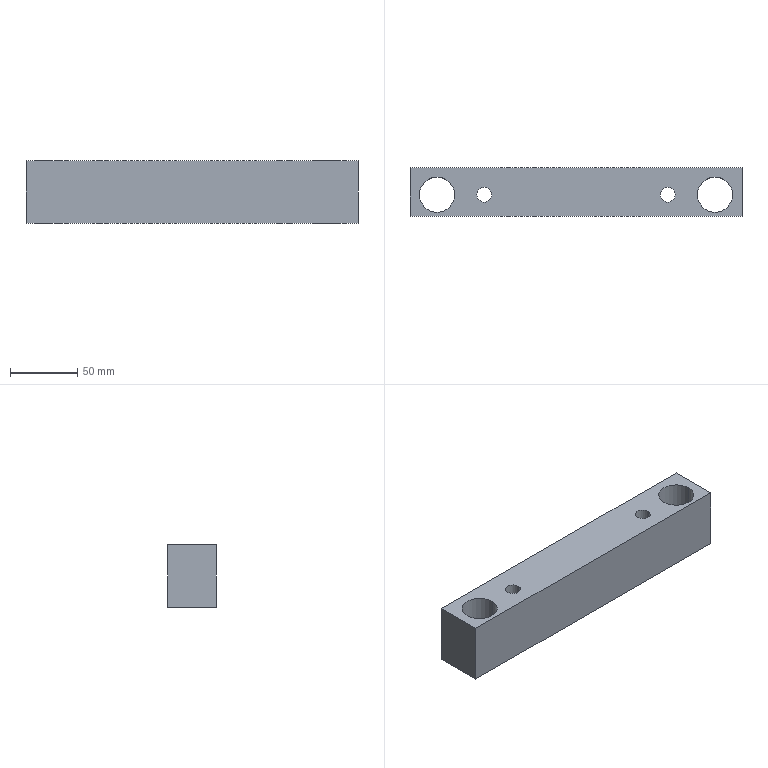Part | STEP file | 5 | 1 solid | 14 faces | box 246 x 36 x 46 mm | volume 349787 mm3 | cylinder 8 | plane 6 | commonest cylinder face diameters 11 x4 26 x4
STEP:
#1=CARTESIAN_POINT('',(0.,0.,0.));
#2=DIRECTION('',(0.,0.,1.));
#3=DIRECTION('',(1.,0.,0.));
#4=AXIS2_PLACEMENT_3D('',#1,#2,#3);
#5=CARTESIAN_POINT('',(116.,78.,22.));
#6=VERTEX_POINT('',#5);
#7=CARTESIAN_POINT('',(116.,78.,68.));
#8=VERTEX_POINT('',#7);
#9=CARTESIAN_POINT('',(116.,78.,68.));
#10=DIRECTION('',(0.,0.,1.));
#11=VECTOR('',#10,1.);
#12=LINE('',#9,#11);
#13=CARTESIAN_POINT('',(103.,78.,68.));
#14=DIRECTION('',(0.,0.,1.));
#15=DIRECTION('',(1.,0.,0.));
#16=AXIS2_PLACEMENT_3D('',#13,#14,#15);
#17=CYLINDRICAL_SURFACE('',#16,13.);
#18=CARTESIAN_POINT('',(6.283,0.));
#19=DIRECTION('',(0.,1.));
#20=VECTOR('',#19,1.);
#21=LINE('',#18,#20);
#22=(GEOMETRIC_REPRESENTATION_CONTEXT(2)PARAMETRIC_REPRESENTATION_CONTEXT()REPRESENTATION_CONTEXT('',''));
#23=DEFINITIONAL_REPRESENTATION('',(#21),#22);
#24=PCURVE('',#17,#23);
#25=CARTESIAN_POINT('',(103.,78.,68.));
#26=DIRECTION('',(0.,0.,1.));
#27=DIRECTION('',(1.,0.,0.));
#28=AXIS2_PLACEMENT_3D('',#25,#26,#27);
#29=CYLINDRICAL_SURFACE('',#28,13.);
#30=CARTESIAN_POINT('',(0.,0.));
#31=DIRECTION('',(0.,1.));
#32=VECTOR('',#31,1.);
#33=LINE('',#30,#32);
#34=(GEOMETRIC_REPRESENTATION_CONTEXT(2)PARAMETRIC_REPRESENTATION_CONTEXT()REPRESENTATION_CONTEXT('',''));
#35=DEFINITIONAL_REPRESENTATION('',(#33),#34);
#36=PCURVE('',#29,#35);
#37=SURFACE_CURVE('',#12,(#24,#36),.PCURVE_S1.);
#38=EDGE_CURVE('',#6,#8,#37,.T.);
#39=ORIENTED_EDGE('',*,*,#38,.T.);
#40=CARTESIAN_POINT('',(90.,78.,68.));
#41=VERTEX_POINT('',#40);
#42=CARTESIAN_POINT('',(103.,78.,68.));
#43=DIRECTION('',(0.,0.,-1.));
#44=DIRECTION('',(1.,0.,0.));
#45=AXIS2_PLACEMENT_3D('',#42,#43,#44);
#46=CIRCLE('',#45,13.);
#47=CARTESIAN_POINT('',(6.283,0.));
#48=DIRECTION('',(-1.,0.));
#49=VECTOR('',#48,1.);
#50=LINE('',#47,#49);
#51=(GEOMETRIC_REPRESENTATION_CONTEXT(2)PARAMETRIC_REPRESENTATION_CONTEXT()REPRESENTATION_CONTEXT('',''));
#52=DEFINITIONAL_REPRESENTATION('',(#50),#51);
#53=PCURVE('',#17,#52);
#54=CARTESIAN_POINT('',(0.,0.,68.));
#55=DIRECTION('',(0.,0.,1.));
#56=DIRECTION('',(1.,0.,0.));
#57=AXIS2_PLACEMENT_3D('',#54,#55,#56);
#58=PLANE('',#57);
#59=CARTESIAN_POINT('',(116.,78.));
#60=CARTESIAN_POINT('',(116.,55.483));
#61=CARTESIAN_POINT('',(96.5,66.742));
#62=CARTESIAN_POINT('',(77.,78.));
#63=CARTESIAN_POINT('',(96.5,89.258));
#64=CARTESIAN_POINT('',(116.,100.517));
#65=CARTESIAN_POINT('',(116.,78.));
#66=(BOUNDED_CURVE()B_SPLINE_CURVE(2,(#59,#60,#61,#62,#63,#64,#65),.UNSPECIFIED.,.T.,.F.)B_SPLINE_CURVE_WITH_KNOTS((1,2,2,2,2,1),(-2.094,0.,2.094,4.189,6.283,8.378),.UNSPECIFIED.)CURVE()GEOMETRIC_REPRESENTATION_ITEM()RATIONAL_B_SPLINE_CURVE((1.,0.5,1.,0.5,1.,0.5,1.))REPRESENTATION_ITEM(''));
#67=(GEOMETRIC_REPRESENTATION_CONTEXT(2)PARAMETRIC_REPRESENTATION_CONTEXT()REPRESENTATION_CONTEXT('',''));
#68=DEFINITIONAL_REPRESENTATION('',(#66),#67);
#69=PCURVE('',#58,#68);
#70=SURFACE_CURVE('',#46,(#53,#69),.PCURVE_S1.);
#71=EDGE_CURVE('',#8,#41,#70,.T.);
#72=ORIENTED_EDGE('',*,*,#71,.T.);
#73=CARTESIAN_POINT('',(90.,78.,22.));
#74=VERTEX_POINT('',#73);
#75=CARTESIAN_POINT('',(90.,78.,68.));
#76=DIRECTION('',(0.,0.,1.));
#77=VECTOR('',#76,1.);
#78=LINE('',#75,#77);
#79=CARTESIAN_POINT('',(3.142,0.));
#80=DIRECTION('',(0.,1.));
#81=VECTOR('',#80,1.);
#82=LINE('',#79,#81);
#83=(GEOMETRIC_REPRESENTATION_CONTEXT(2)PARAMETRIC_REPRESENTATION_CONTEXT()REPRESENTATION_CONTEXT('',''));
#84=DEFINITIONAL_REPRESENTATION('',(#82),#83);
#85=PCURVE('',#17,#84);
#86=CARTESIAN_POINT('',(3.142,0.));
#87=DIRECTION('',(0.,1.));
#88=VECTOR('',#87,1.);
#89=LINE('',#86,#88);
#90=(GEOMETRIC_REPRESENTATION_CONTEXT(2)PARAMETRIC_REPRESENTATION_CONTEXT()REPRESENTATION_CONTEXT('',''));
#91=DEFINITIONAL_REPRESENTATION('',(#89),#90);
#92=PCURVE('',#29,#91);
#93=SURFACE_CURVE('',#78,(#85,#92),.PCURVE_S1.);
#94=EDGE_CURVE('',#74,#41,#93,.T.);
#95=ORIENTED_EDGE('',*,*,#94,.F.);
#96=CARTESIAN_POINT('',(103.,78.,22.));
#97=DIRECTION('',(0.,0.,-1.));
#98=DIRECTION('',(1.,0.,0.));
#99=AXIS2_PLACEMENT_3D('',#96,#97,#98);
#100=CIRCLE('',#99,13.);
#101=CARTESIAN_POINT('',(6.283,-46.));
#102=DIRECTION('',(-1.,0.));
#103=VECTOR('',#102,1.);
#104=LINE('',#101,#103);
#105=(GEOMETRIC_REPRESENTATION_CONTEXT(2)PARAMETRIC_REPRESENTATION_CONTEXT()REPRESENTATION_CONTEXT('',''));
#106=DEFINITIONAL_REPRESENTATION('',(#104),#105);
#107=PCURVE('',#17,#106);
#108=CARTESIAN_POINT('',(0.,0.,22.));
#109=DIRECTION('',(0.,0.,1.));
#110=DIRECTION('',(1.,0.,0.));
#111=AXIS2_PLACEMENT_3D('',#108,#109,#110);
#112=PLANE('',#111);
#113=CARTESIAN_POINT('',(116.,78.));
#114=CARTESIAN_POINT('',(116.,55.483));
#115=CARTESIAN_POINT('',(96.5,66.742));
#116=CARTESIAN_POINT('',(77.,78.));
#117=CARTESIAN_POINT('',(96.5,89.258));
#118=CARTESIAN_POINT('',(116.,100.517));
#119=CARTESIAN_POINT('',(116.,78.));
#120=(BOUNDED_CURVE()B_SPLINE_CURVE(2,(#113,#114,#115,#116,#117,#118,#119),.UNSPECIFIED.,.T.,.F.)B_SPLINE_CURVE_WITH_KNOTS((1,2,2,2,2,1),(-2.094,0.,2.094,4.189,6.283,8.378),.UNSPECIFIED.)CURVE()GEOMETRIC_REPRESENTATION_ITEM()RATIONAL_B_SPLINE_CURVE((1.,0.5,1.,0.5,1.,0.5,1.))REPRESENTATION_ITEM(''));
#121=(GEOMETRIC_REPRESENTATION_CONTEXT(2)PARAMETRIC_REPRESENTATION_CONTEXT()REPRESENTATION_CONTEXT('',''));
#122=DEFINITIONAL_REPRESENTATION('',(#120),#121);
#123=PCURVE('',#112,#122);
#124=SURFACE_CURVE('',#100,(#107,#123),.PCURVE_S1.);
#125=EDGE_CURVE('',#6,#74,#124,.T.);
#126=ORIENTED_EDGE('',*,*,#125,.F.);
#127=EDGE_LOOP('',(#39,#72,#95,#126));
#128=FACE_BOUND('',#127,.F.);
#129=ADVANCED_FACE('',(#128),#17,.F.);
#130=CARTESIAN_POINT('',(-90.,78.,22.));
#131=VERTEX_POINT('',#130);
#132=CARTESIAN_POINT('',(-90.,78.,68.));
#133=VERTEX_POINT('',#132);
#134=CARTESIAN_POINT('',(-90.,78.,68.));
#135=DIRECTION('',(0.,0.,1.));
#136=VECTOR('',#135,1.);
#137=LINE('',#134,#136);
#138=CARTESIAN_POINT('',(-103.,78.,68.));
#139=DIRECTION('',(0.,0.,1.));
#140=DIRECTION('',(1.,0.,0.));
#141=AXIS2_PLACEMENT_3D('',#138,#139,#140);
#142=CYLINDRICAL_SURFACE('',#141,13.);
#143=CARTESIAN_POINT('',(6.283,0.));
#144=DIRECTION('',(0.,1.));
#145=VECTOR('',#144,1.);
#146=LINE('',#143,#145);
#147=(GEOMETRIC_REPRESENTATION_CONTEXT(2)PARAMETRIC_REPRESENTATION_CONTEXT()REPRESENTATION_CONTEXT('',''));
#148=DEFINITIONAL_REPRESENTATION('',(#146),#147);
#149=PCURVE('',#142,#148);
#150=CARTESIAN_POINT('',(-103.,78.,68.));
#151=DIRECTION('',(0.,0.,1.));
#152=DIRECTION('',(1.,0.,0.));
#153=AXIS2_PLACEMENT_3D('',#150,#151,#152);
#154=CYLINDRICAL_SURFACE('',#153,13.);
#155=CARTESIAN_POINT('',(0.,0.));
#156=DIRECTION('',(0.,1.));
#157=VECTOR('',#156,1.);
#158=LINE('',#155,#157);
#159=(GEOMETRIC_REPRESENTATION_CONTEXT(2)PARAMETRIC_REPRESENTATION_CONTEXT()REPRESENTATION_CONTEXT('',''));
#160=DEFINITIONAL_REPRESENTATION('',(#158),#159);
#161=PCURVE('',#154,#160);
#162=SURFACE_CURVE('',#137,(#149,#161),.PCURVE_S1.);
#163=EDGE_CURVE('',#131,#133,#162,.T.);
#164=ORIENTED_EDGE('',*,*,#163,.T.);
#165=CARTESIAN_POINT('',(-116.,78.,68.));
#166=VERTEX_POINT('',#165);
#167=CARTESIAN_POINT('',(-103.,78.,68.));
#168=DIRECTION('',(0.,0.,-1.));
#169=DIRECTION('',(1.,0.,0.));
#170=AXIS2_PLACEMENT_3D('',#167,#168,#169);
#171=CIRCLE('',#170,13.);
#172=CARTESIAN_POINT('',(6.283,0.));
#173=DIRECTION('',(-1.,0.));
#174=VECTOR('',#173,1.);
#175=LINE('',#172,#174);
#176=(GEOMETRIC_REPRESENTATION_CONTEXT(2)PARAMETRIC_REPRESENTATION_CONTEXT()REPRESENTATION_CONTEXT('',''));
#177=DEFINITIONAL_REPRESENTATION('',(#175),#176);
#178=PCURVE('',#142,#177);
#179=CARTESIAN_POINT('',(-90.,78.));
#180=CARTESIAN_POINT('',(-90.,55.483));
#181=CARTESIAN_POINT('',(-109.5,66.742));
#182=CARTESIAN_POINT('',(-129.,78.));
#183=CARTESIAN_POINT('',(-109.5,89.258));
#184=CARTESIAN_POINT('',(-90.,100.517));
#185=CARTESIAN_POINT('',(-90.,78.));
#186=(BOUNDED_CURVE()B_SPLINE_CURVE(2,(#179,#180,#181,#182,#183,#184,#185),.UNSPECIFIED.,.T.,.F.)B_SPLINE_CURVE_WITH_KNOTS((1,2,2,2,2,1),(-2.094,0.,2.094,4.189,6.283,8.378),.UNSPECIFIED.)CURVE()GEOMETRIC_REPRESENTATION_ITEM()RATIONAL_B_SPLINE_CURVE((1.,0.5,1.,0.5,1.,0.5,1.))REPRESENTATION_ITEM(''));
#187=(GEOMETRIC_REPRESENTATION_CONTEXT(2)PARAMETRIC_REPRESENTATION_CONTEXT()REPRESENTATION_CONTEXT('',''));
#188=DEFINITIONAL_REPRESENTATION('',(#186),#187);
#189=PCURVE('',#58,#188);
#190=SURFACE_CURVE('',#171,(#178,#189),.PCURVE_S1.);
#191=EDGE_CURVE('',#133,#166,#190,.T.);
#192=ORIENTED_EDGE('',*,*,#191,.T.);
#193=CARTESIAN_POINT('',(-116.,78.,22.));
#194=VERTEX_POINT('',#193);
#195=CARTESIAN_POINT('',(-116.,78.,68.));
#196=DIRECTION('',(0.,0.,1.));
#197=VECTOR('',#196,1.);
#198=LINE('',#195,#197);
#199=CARTESIAN_POINT('',(3.142,0.));
#200=DIRECTION('',(0.,1.));
#201=VECTOR('',#200,1.);
#202=LINE('',#199,#201);
#203=(GEOMETRIC_REPRESENTATION_CONTEXT(2)PARAMETRIC_REPRESENTATION_CONTEXT()REPRESENTATION_CONTEXT('',''));
#204=DEFINITIONAL_REPRESENTATION('',(#202),#203);
#205=PCURVE('',#142,#204);
#206=CARTESIAN_POINT('',(3.142,0.));
#207=DIRECTION('',(0.,1.));
#208=VECTOR('',#207,1.);
#209=LINE('',#206,#208);
#210=(GEOMETRIC_REPRESENTATION_CONTEXT(2)PARAMETRIC_REPRESENTATION_CONTEXT()REPRESENTATION_CONTEXT('',''));
#211=DEFINITIONAL_REPRESENTATION('',(#209),#210);
#212=PCURVE('',#154,#211);
#213=SURFACE_CURVE('',#198,(#205,#212),.PCURVE_S1.);
#214=EDGE_CURVE('',#194,#166,#213,.T.);
#215=ORIENTED_EDGE('',*,*,#214,.F.);
#216=CARTESIAN_POINT('',(-103.,78.,22.));
#217=DIRECTION('',(0.,0.,-1.));
#218=DIRECTION('',(1.,0.,0.));
#219=AXIS2_PLACEMENT_3D('',#216,#217,#218);
#220=CIRCLE('',#219,13.);
#221=CARTESIAN_POINT('',(6.283,-46.));
#222=DIRECTION('',(-1.,0.));
#223=VECTOR('',#222,1.);
#224=LINE('',#221,#223);
#225=(GEOMETRIC_REPRESENTATION_CONTEXT(2)PARAMETRIC_REPRESENTATION_CONTEXT()REPRESENTATION_CONTEXT('',''));
#226=DEFINITIONAL_REPRESENTATION('',(#224),#225);
#227=PCURVE('',#142,#226);
#228=CARTESIAN_POINT('',(-90.,78.));
#229=CARTESIAN_POINT('',(-90.,55.483));
#230=CARTESIAN_POINT('',(-109.5,66.742));
#231=CARTESIAN_POINT('',(-129.,78.));
#232=CARTESIAN_POINT('',(-109.5,89.258));
#233=CARTESIAN_POINT('',(-90.,100.517));
#234=CARTESIAN_POINT('',(-90.,78.));
#235=(BOUNDED_CURVE()B_SPLINE_CURVE(2,(#228,#229,#230,#231,#232,#233,#234),.UNSPECIFIED.,.T.,.F.)B_SPLINE_CURVE_WITH_KNOTS((1,2,2,2,2,1),(-2.094,0.,2.094,4.189,6.283,8.378),.UNSPECIFIED.)CURVE()GEOMETRIC_REPRESENTATION_ITEM()RATIONAL_B_SPLINE_CURVE((1.,0.5,1.,0.5,1.,0.5,1.))REPRESENTATION_ITEM(''));
#236=(GEOMETRIC_REPRESENTATION_CONTEXT(2)PARAMETRIC_REPRESENTATION_CONTEXT()REPRESENTATION_CONTEXT('',''));
#237=DEFINITIONAL_REPRESENTATION('',(#235),#236);
#238=PCURVE('',#112,#237);
#239=SURFACE_CURVE('',#220,(#227,#238),.PCURVE_S1.);
#240=EDGE_CURVE('',#131,#194,#239,.T.);
#241=ORIENTED_EDGE('',*,*,#240,.F.);
#242=EDGE_LOOP('',(#164,#192,#215,#241));
#243=FACE_BOUND('',#242,.F.);
#244=ADVANCED_FACE('',(#243),#142,.F.);
#245=CARTESIAN_POINT('',(62.5,78.,68.));
#246=VERTEX_POINT('',#245);
#247=CARTESIAN_POINT('',(62.5,78.,22.));
#248=VERTEX_POINT('',#247);
#249=CARTESIAN_POINT('',(62.5,78.,45.));
#250=DIRECTION('',(0.,0.,-1.));
#251=VECTOR('',#250,1.);
#252=LINE('',#249,#251);
#253=CARTESIAN_POINT('',(68.,78.,45.));
#254=DIRECTION('',(0.,0.,-1.));
#255=DIRECTION('',(-1.,0.,0.));
#256=AXIS2_PLACEMENT_3D('',#253,#254,#255);
#257=CYLINDRICAL_SURFACE('',#256,5.5);
#258=CARTESIAN_POINT('',(6.283,0.));
#259=DIRECTION('',(0.,1.));
#260=VECTOR('',#259,1.);
#261=LINE('',#258,#260);
#262=(GEOMETRIC_REPRESENTATION_CONTEXT(2)PARAMETRIC_REPRESENTATION_CONTEXT()REPRESENTATION_CONTEXT('',''));
#263=DEFINITIONAL_REPRESENTATION('',(#261),#262);
#264=PCURVE('',#257,#263);
#265=CARTESIAN_POINT('',(68.,78.,45.));
#266=DIRECTION('',(0.,0.,-1.));
#267=DIRECTION('',(-1.,0.,0.));
#268=AXIS2_PLACEMENT_3D('',#265,#266,#267);
#269=CYLINDRICAL_SURFACE('',#268,5.5);
#270=CARTESIAN_POINT('',(0.,0.));
#271=DIRECTION('',(0.,1.));
#272=VECTOR('',#271,1.);
#273=LINE('',#270,#272);
#274=(GEOMETRIC_REPRESENTATION_CONTEXT(2)PARAMETRIC_REPRESENTATION_CONTEXT()REPRESENTATION_CONTEXT('',''));
#275=DEFINITIONAL_REPRESENTATION('',(#273),#274);
#276=PCURVE('',#269,#275);
#277=SURFACE_CURVE('',#252,(#264,#276),.PCURVE_S1.);
#278=EDGE_CURVE('',#246,#248,#277,.T.);
#279=ORIENTED_EDGE('',*,*,#278,.T.);
#280=CARTESIAN_POINT('',(73.5,78.,22.));
#281=VERTEX_POINT('',#280);
#282=CARTESIAN_POINT('',(68.,78.,22.));
#283=DIRECTION('',(0.,0.,-1.));
#284=DIRECTION('',(-1.,0.,0.));
#285=AXIS2_PLACEMENT_3D('',#282,#283,#284);
#286=CIRCLE('',#285,5.5);
#287=CARTESIAN_POINT('',(0.,23.));
#288=DIRECTION('',(1.,0.));
#289=VECTOR('',#288,1.);
#290=LINE('',#287,#289);
#291=(GEOMETRIC_REPRESENTATION_CONTEXT(2)PARAMETRIC_REPRESENTATION_CONTEXT()REPRESENTATION_CONTEXT('',''));
#292=DEFINITIONAL_REPRESENTATION('',(#290),#291);
#293=PCURVE('',#257,#292);
#294=CARTESIAN_POINT('',(62.5,78.));
#295=CARTESIAN_POINT('',(62.5,87.526));
#296=CARTESIAN_POINT('',(70.75,82.763));
#297=CARTESIAN_POINT('',(79.,78.));
#298=CARTESIAN_POINT('',(70.75,73.237));
#299=CARTESIAN_POINT('',(62.5,68.474));
#300=CARTESIAN_POINT('',(62.5,78.));
#301=(BOUNDED_CURVE()B_SPLINE_CURVE(2,(#294,#295,#296,#297,#298,#299,#300),.UNSPECIFIED.,.T.,.F.)B_SPLINE_CURVE_WITH_KNOTS((1,2,2,2,2,1),(-2.094,0.,2.094,4.189,6.283,8.378),.UNSPECIFIED.)CURVE()GEOMETRIC_REPRESENTATION_ITEM()RATIONAL_B_SPLINE_CURVE((1.,0.5,1.,0.5,1.,0.5,1.))REPRESENTATION_ITEM(''));
#302=(GEOMETRIC_REPRESENTATION_CONTEXT(2)PARAMETRIC_REPRESENTATION_CONTEXT()REPRESENTATION_CONTEXT('',''));
#303=DEFINITIONAL_REPRESENTATION('',(#301),#302);
#304=PCURVE('',#112,#303);
#305=SURFACE_CURVE('',#286,(#293,#304),.PCURVE_S1.);
#306=EDGE_CURVE('',#281,#248,#305,.T.);
#307=ORIENTED_EDGE('',*,*,#306,.F.);
#308=CARTESIAN_POINT('',(73.5,78.,68.));
#309=VERTEX_POINT('',#308);
#310=CARTESIAN_POINT('',(73.5,78.,45.));
#311=DIRECTION('',(0.,0.,-1.));
#312=VECTOR('',#311,1.);
#313=LINE('',#310,#312);
#314=CARTESIAN_POINT('',(3.142,0.));
#315=DIRECTION('',(0.,1.));
#316=VECTOR('',#315,1.);
#317=LINE('',#314,#316);
#318=(GEOMETRIC_REPRESENTATION_CONTEXT(2)PARAMETRIC_REPRESENTATION_CONTEXT()REPRESENTATION_CONTEXT('',''));
#319=DEFINITIONAL_REPRESENTATION('',(#317),#318);
#320=PCURVE('',#257,#319);
#321=CARTESIAN_POINT('',(3.142,0.));
#322=DIRECTION('',(0.,1.));
#323=VECTOR('',#322,1.);
#324=LINE('',#321,#323);
#325=(GEOMETRIC_REPRESENTATION_CONTEXT(2)PARAMETRIC_REPRESENTATION_CONTEXT()REPRESENTATION_CONTEXT('',''));
#326=DEFINITIONAL_REPRESENTATION('',(#324),#325);
#327=PCURVE('',#269,#326);
#328=SURFACE_CURVE('',#313,(#320,#327),.PCURVE_S1.);
#329=EDGE_CURVE('',#309,#281,#328,.T.);
#330=ORIENTED_EDGE('',*,*,#329,.F.);
#331=CARTESIAN_POINT('',(68.,78.,68.));
#332=DIRECTION('',(0.,0.,-1.));
#333=DIRECTION('',(-1.,0.,0.));
#334=AXIS2_PLACEMENT_3D('',#331,#332,#333);
#335=CIRCLE('',#334,5.5);
#336=CARTESIAN_POINT('',(0.,-23.));
#337=DIRECTION('',(1.,0.));
#338=VECTOR('',#337,1.);
#339=LINE('',#336,#338);
#340=(GEOMETRIC_REPRESENTATION_CONTEXT(2)PARAMETRIC_REPRESENTATION_CONTEXT()REPRESENTATION_CONTEXT('',''));
#341=DEFINITIONAL_REPRESENTATION('',(#339),#340);
#342=PCURVE('',#257,#341);
#343=CARTESIAN_POINT('',(62.5,78.));
#344=CARTESIAN_POINT('',(62.5,87.526));
#345=CARTESIAN_POINT('',(70.75,82.763));
#346=CARTESIAN_POINT('',(79.,78.));
#347=CARTESIAN_POINT('',(70.75,73.237));
#348=CARTESIAN_POINT('',(62.5,68.474));
#349=CARTESIAN_POINT('',(62.5,78.));
#350=(BOUNDED_CURVE()B_SPLINE_CURVE(2,(#343,#344,#345,#346,#347,#348,#349),.UNSPECIFIED.,.T.,.F.)B_SPLINE_CURVE_WITH_KNOTS((1,2,2,2,2,1),(-2.094,0.,2.094,4.189,6.283,8.378),.UNSPECIFIED.)CURVE()GEOMETRIC_REPRESENTATION_ITEM()RATIONAL_B_SPLINE_CURVE((1.,0.5,1.,0.5,1.,0.5,1.))REPRESENTATION_ITEM(''));
#351=(GEOMETRIC_REPRESENTATION_CONTEXT(2)PARAMETRIC_REPRESENTATION_CONTEXT()REPRESENTATION_CONTEXT('',''));
#352=DEFINITIONAL_REPRESENTATION('',(#350),#351);
#353=PCURVE('',#58,#352);
#354=SURFACE_CURVE('',#335,(#342,#353),.PCURVE_S1.);
#355=EDGE_CURVE('',#309,#246,#354,.T.);
#356=ORIENTED_EDGE('',*,*,#355,.T.);
#357=EDGE_LOOP('',(#279,#307,#330,#356));
#358=FACE_BOUND('',#357,.F.);
#359=ADVANCED_FACE('',(#358),#257,.F.);
#360=CARTESIAN_POINT('',(-73.5,78.,68.));
#361=VERTEX_POINT('',#360);
#362=CARTESIAN_POINT('',(-73.5,78.,22.));
#363=VERTEX_POINT('',#362);
#364=CARTESIAN_POINT('',(-73.5,78.,45.));
#365=DIRECTION('',(0.,0.,-1.));
#366=VECTOR('',#365,1.);
#367=LINE('',#364,#366);
#368=CARTESIAN_POINT('',(-68.,78.,45.));
#369=DIRECTION('',(0.,0.,-1.));
#370=DIRECTION('',(-1.,0.,0.));
#371=AXIS2_PLACEMENT_3D('',#368,#369,#370);
#372=CYLINDRICAL_SURFACE('',#371,5.5);
#373=CARTESIAN_POINT('',(6.283,0.));
#374=DIRECTION('',(0.,1.));
#375=VECTOR('',#374,1.);
#376=LINE('',#373,#375);
#377=(GEOMETRIC_REPRESENTATION_CONTEXT(2)PARAMETRIC_REPRESENTATION_CONTEXT()REPRESENTATION_CONTEXT('',''));
#378=DEFINITIONAL_REPRESENTATION('',(#376),#377);
#379=PCURVE('',#372,#378);
#380=CARTESIAN_POINT('',(-68.,78.,45.));
#381=DIRECTION('',(0.,0.,-1.));
#382=DIRECTION('',(-1.,0.,0.));
#383=AXIS2_PLACEMENT_3D('',#380,#381,#382);
#384=CYLINDRICAL_SURFACE('',#383,5.5);
#385=CARTESIAN_POINT('',(0.,0.));
#386=DIRECTION('',(0.,1.));
#387=VECTOR('',#386,1.);
#388=LINE('',#385,#387);
#389=(GEOMETRIC_REPRESENTATION_CONTEXT(2)PARAMETRIC_REPRESENTATION_CONTEXT()REPRESENTATION_CONTEXT('',''));
#390=DEFINITIONAL_REPRESENTATION('',(#388),#389);
#391=PCURVE('',#384,#390);
#392=SURFACE_CURVE('',#367,(#379,#391),.PCURVE_S1.);
#393=EDGE_CURVE('',#361,#363,#392,.T.);
#394=ORIENTED_EDGE('',*,*,#393,.T.);
#395=CARTESIAN_POINT('',(-62.5,78.,22.));
#396=VERTEX_POINT('',#395);
#397=CARTESIAN_POINT('',(-68.,78.,22.));
#398=DIRECTION('',(0.,0.,-1.));
#399=DIRECTION('',(-1.,0.,0.));
#400=AXIS2_PLACEMENT_3D('',#397,#398,#399);
#401=CIRCLE('',#400,5.5);
#402=CARTESIAN_POINT('',(0.,23.));
#403=DIRECTION('',(1.,0.));
#404=VECTOR('',#403,1.);
#405=LINE('',#402,#404);
#406=(GEOMETRIC_REPRESENTATION_CONTEXT(2)PARAMETRIC_REPRESENTATION_CONTEXT()REPRESENTATION_CONTEXT('',''));
#407=DEFINITIONAL_REPRESENTATION('',(#405),#406);
#408=PCURVE('',#372,#407);
#409=CARTESIAN_POINT('',(-73.5,78.));
#410=CARTESIAN_POINT('',(-73.5,87.526));
#411=CARTESIAN_POINT('',(-65.25,82.763));
#412=CARTESIAN_POINT('',(-57.,78.));
#413=CARTESIAN_POINT('',(-65.25,73.237));
#414=CARTESIAN_POINT('',(-73.5,68.474));
#415=CARTESIAN_POINT('',(-73.5,78.));
#416=(BOUNDED_CURVE()B_SPLINE_CURVE(2,(#409,#410,#411,#412,#413,#414,#415),.UNSPECIFIED.,.T.,.F.)B_SPLINE_CURVE_WITH_KNOTS((1,2,2,2,2,1),(-2.094,0.,2.094,4.189,6.283,8.378),.UNSPECIFIED.)CURVE()GEOMETRIC_REPRESENTATION_ITEM()RATIONAL_B_SPLINE_CURVE((1.,0.5,1.,0.5,1.,0.5,1.))REPRESENTATION_ITEM(''));
#417=(GEOMETRIC_REPRESENTATION_CONTEXT(2)PARAMETRIC_REPRESENTATION_CONTEXT()REPRESENTATION_CONTEXT('',''));
#418=DEFINITIONAL_REPRESENTATION('',(#416),#417);
#419=PCURVE('',#112,#418);
#420=SURFACE_CURVE('',#401,(#408,#419),.PCURVE_S1.);
#421=EDGE_CURVE('',#396,#363,#420,.T.);
#422=ORIENTED_EDGE('',*,*,#421,.F.);
#423=CARTESIAN_POINT('',(-62.5,78.,68.));
#424=VERTEX_POINT('',#423);
#425=CARTESIAN_POINT('',(-62.5,78.,45.));
#426=DIRECTION('',(0.,0.,-1.));
#427=VECTOR('',#426,1.);
#428=LINE('',#425,#427);
#429=CARTESIAN_POINT('',(3.142,0.));
#430=DIRECTION('',(0.,1.));
#431=VECTOR('',#430,1.);
#432=LINE('',#429,#431);
#433=(GEOMETRIC_REPRESENTATION_CONTEXT(2)PARAMETRIC_REPRESENTATION_CONTEXT()REPRESENTATION_CONTEXT('',''));
#434=DEFINITIONAL_REPRESENTATION('',(#432),#433);
#435=PCURVE('',#372,#434);
#436=CARTESIAN_POINT('',(3.142,0.));
#437=DIRECTION('',(0.,1.));
#438=VECTOR('',#437,1.);
#439=LINE('',#436,#438);
#440=(GEOMETRIC_REPRESENTATION_CONTEXT(2)PARAMETRIC_REPRESENTATION_CONTEXT()REPRESENTATION_CONTEXT('',''));
#441=DEFINITIONAL_REPRESENTATION('',(#439),#440);
#442=PCURVE('',#384,#441);
#443=SURFACE_CURVE('',#428,(#435,#442),.PCURVE_S1.);
#444=EDGE_CURVE('',#424,#396,#443,.T.);
#445=ORIENTED_EDGE('',*,*,#444,.F.);
#446=CARTESIAN_POINT('',(-68.,78.,68.));
#447=DIRECTION('',(0.,0.,-1.));
#448=DIRECTION('',(-1.,0.,0.));
#449=AXIS2_PLACEMENT_3D('',#446,#447,#448);
#450=CIRCLE('',#449,5.5);
#451=CARTESIAN_POINT('',(0.,-23.));
#452=DIRECTION('',(1.,0.));
#453=VECTOR('',#452,1.);
#454=LINE('',#451,#453);
#455=(GEOMETRIC_REPRESENTATION_CONTEXT(2)PARAMETRIC_REPRESENTATION_CONTEXT()REPRESENTATION_CONTEXT('',''));
#456=DEFINITIONAL_REPRESENTATION('',(#454),#455);
#457=PCURVE('',#372,#456);
#458=CARTESIAN_POINT('',(-73.5,78.));
#459=CARTESIAN_POINT('',(-73.5,87.526));
#460=CARTESIAN_POINT('',(-65.25,82.763));
#461=CARTESIAN_POINT('',(-57.,78.));
#462=CARTESIAN_POINT('',(-65.25,73.237));
#463=CARTESIAN_POINT('',(-73.5,68.474));
#464=CARTESIAN_POINT('',(-73.5,78.));
#465=(BOUNDED_CURVE()B_SPLINE_CURVE(2,(#458,#459,#460,#461,#462,#463,#464),.UNSPECIFIED.,.T.,.F.)B_SPLINE_CURVE_WITH_KNOTS((1,2,2,2,2,1),(-2.094,0.,2.094,4.189,6.283,8.378),.UNSPECIFIED.)CURVE()GEOMETRIC_REPRESENTATION_ITEM()RATIONAL_B_SPLINE_CURVE((1.,0.5,1.,0.5,1.,0.5,1.))REPRESENTATION_ITEM(''));
#466=(GEOMETRIC_REPRESENTATION_CONTEXT(2)PARAMETRIC_REPRESENTATION_CONTEXT()REPRESENTATION_CONTEXT('',''));
#467=DEFINITIONAL_REPRESENTATION('',(#465),#466);
#468=PCURVE('',#58,#467);
#469=SURFACE_CURVE('',#450,(#457,#468),.PCURVE_S1.);
#470=EDGE_CURVE('',#424,#361,#469,.T.);
#471=ORIENTED_EDGE('',*,*,#470,.T.);
#472=EDGE_LOOP('',(#394,#422,#445,#471));
#473=FACE_BOUND('',#472,.F.);
#474=ADVANCED_FACE('',(#473),#372,.F.);
#475=CARTESIAN_POINT('',(123.,98.,22.));
#476=VERTEX_POINT('',#475);
#477=CARTESIAN_POINT('',(-123.,98.,22.));
#478=VERTEX_POINT('',#477);
#479=CARTESIAN_POINT('',(-123.,98.,22.));
#480=DIRECTION('',(-1.,0.,0.));
#481=VECTOR('',#480,1.);
#482=LINE('',#479,#481);
#483=CARTESIAN_POINT('',(-123.,98.,22.));
#484=DIRECTION('',(0.,1.,0.));
#485=DIRECTION('',(0.,0.,1.));
#486=AXIS2_PLACEMENT_3D('',#483,#484,#485);
#487=PLANE('',#486);
#488=CARTESIAN_POINT('',(0.,0.));
#489=DIRECTION('',(0.,-1.));
#490=VECTOR('',#489,1.);
#491=LINE('',#488,#490);
#492=(GEOMETRIC_REPRESENTATION_CONTEXT(2)PARAMETRIC_REPRESENTATION_CONTEXT()REPRESENTATION_CONTEXT('',''));
#493=DEFINITIONAL_REPRESENTATION('',(#491),#492);
#494=PCURVE('',#487,#493);
#495=CARTESIAN_POINT('',(-123.,98.));
#496=DIRECTION('',(-1.,0.));
#497=VECTOR('',#496,1.);
#498=LINE('',#495,#497);
#499=(GEOMETRIC_REPRESENTATION_CONTEXT(2)PARAMETRIC_REPRESENTATION_CONTEXT()REPRESENTATION_CONTEXT('',''));
#500=DEFINITIONAL_REPRESENTATION('',(#498),#499);
#501=PCURVE('',#112,#500);
#502=SURFACE_CURVE('',#482,(#494,#501),.PCURVE_S1.);
#503=EDGE_CURVE('',#476,#478,#502,.T.);
#504=ORIENTED_EDGE('',*,*,#503,.T.);
#505=CARTESIAN_POINT('',(-123.,98.,68.));
#506=VERTEX_POINT('',#505);
#507=CARTESIAN_POINT('',(-123.,98.,22.));
#508=DIRECTION('',(0.,0.,1.));
#509=VECTOR('',#508,1.);
#510=LINE('',#507,#509);
#511=CARTESIAN_POINT('',(0.,0.));
#512=DIRECTION('',(1.,0.));
#513=VECTOR('',#512,1.);
#514=LINE('',#511,#513);
#515=(GEOMETRIC_REPRESENTATION_CONTEXT(2)PARAMETRIC_REPRESENTATION_CONTEXT()REPRESENTATION_CONTEXT('',''));
#516=DEFINITIONAL_REPRESENTATION('',(#514),#515);
#517=PCURVE('',#487,#516);
#518=CARTESIAN_POINT('',(-123.,62.,22.));
#519=DIRECTION('',(-1.,0.,0.));
#520=DIRECTION('',(0.,0.,1.));
#521=AXIS2_PLACEMENT_3D('',#518,#519,#520);
#522=PLANE('',#521);
#523=CARTESIAN_POINT('',(0.,36.));
#524=DIRECTION('',(1.,0.));
#525=VECTOR('',#524,1.);
#526=LINE('',#523,#525);
#527=(GEOMETRIC_REPRESENTATION_CONTEXT(2)PARAMETRIC_REPRESENTATION_CONTEXT()REPRESENTATION_CONTEXT('',''));
#528=DEFINITIONAL_REPRESENTATION('',(#526),#527);
#529=PCURVE('',#522,#528);
#530=SURFACE_CURVE('',#510,(#517,#529),.PCURVE_S1.);
#531=EDGE_CURVE('',#478,#506,#530,.T.);
#532=ORIENTED_EDGE('',*,*,#531,.T.);
#533=CARTESIAN_POINT('',(123.,98.,68.));
#534=VERTEX_POINT('',#533);
#535=CARTESIAN_POINT('',(-123.,98.,68.));
#536=DIRECTION('',(1.,0.,0.));
#537=VECTOR('',#536,1.);
#538=LINE('',#535,#537);
#539=CARTESIAN_POINT('',(46.,0.));
#540=DIRECTION('',(0.,1.));
#541=VECTOR('',#540,1.);
#542=LINE('',#539,#541);
#543=(GEOMETRIC_REPRESENTATION_CONTEXT(2)PARAMETRIC_REPRESENTATION_CONTEXT()REPRESENTATION_CONTEXT('',''));
#544=DEFINITIONAL_REPRESENTATION('',(#542),#543);
#545=PCURVE('',#487,#544);
#546=CARTESIAN_POINT('',(-123.,98.));
#547=DIRECTION('',(1.,0.));
#548=VECTOR('',#547,1.);
#549=LINE('',#546,#548);
#550=(GEOMETRIC_REPRESENTATION_CONTEXT(2)PARAMETRIC_REPRESENTATION_CONTEXT()REPRESENTATION_CONTEXT('',''));
#551=DEFINITIONAL_REPRESENTATION('',(#549),#550);
#552=PCURVE('',#58,#551);
#553=SURFACE_CURVE('',#538,(#545,#552),.PCURVE_S1.);
#554=EDGE_CURVE('',#506,#534,#553,.T.);
#555=ORIENTED_EDGE('',*,*,#554,.T.);
#556=CARTESIAN_POINT('',(123.,98.,22.));
#557=DIRECTION('',(0.,0.,-1.));
#558=VECTOR('',#557,1.);
#559=LINE('',#556,#558);
#560=CARTESIAN_POINT('',(0.,246.));
#561=DIRECTION('',(-1.,0.));
#562=VECTOR('',#561,1.);
#563=LINE('',#560,#562);
#564=(GEOMETRIC_REPRESENTATION_CONTEXT(2)PARAMETRIC_REPRESENTATION_CONTEXT()REPRESENTATION_CONTEXT('',''));
#565=DEFINITIONAL_REPRESENTATION('',(#563),#564);
#566=PCURVE('',#487,#565);
#567=CARTESIAN_POINT('',(123.,98.,22.));
#568=DIRECTION('',(1.,0.,0.));
#569=DIRECTION('',(0.,0.,-1.));
#570=AXIS2_PLACEMENT_3D('',#567,#568,#569);
#571=PLANE('',#570);
#572=CARTESIAN_POINT('',(0.,0.));
#573=DIRECTION('',(1.,0.));
#574=VECTOR('',#573,1.);
#575=LINE('',#572,#574);
#576=(GEOMETRIC_REPRESENTATION_CONTEXT(2)PARAMETRIC_REPRESENTATION_CONTEXT()REPRESENTATION_CONTEXT('',''));
#577=DEFINITIONAL_REPRESENTATION('',(#575),#576);
#578=PCURVE('',#571,#577);
#579=SURFACE_CURVE('',#559,(#566,#578),.PCURVE_S1.);
#580=EDGE_CURVE('',#534,#476,#579,.T.);
#581=ORIENTED_EDGE('',*,*,#580,.T.);
#582=EDGE_LOOP('',(#504,#532,#555,#581));
#583=FACE_BOUND('',#582,.T.);
#584=ADVANCED_FACE('',(#583),#487,.T.);
#585=CARTESIAN_POINT('',(-123.,62.,22.));
#586=VERTEX_POINT('',#585);
#587=CARTESIAN_POINT('',(-123.,62.,22.));
#588=DIRECTION('',(0.,-1.,0.));
#589=VECTOR('',#588,1.);
#590=LINE('',#587,#589);
#591=CARTESIAN_POINT('',(0.,0.));
#592=DIRECTION('',(0.,-1.));
#593=VECTOR('',#592,1.);
#594=LINE('',#591,#593);
#595=(GEOMETRIC_REPRESENTATION_CONTEXT(2)PARAMETRIC_REPRESENTATION_CONTEXT()REPRESENTATION_CONTEXT('',''));
#596=DEFINITIONAL_REPRESENTATION('',(#594),#595);
#597=PCURVE('',#522,#596);
#598=CARTESIAN_POINT('',(-123.,62.));
#599=DIRECTION('',(0.,-1.));
#600=VECTOR('',#599,1.);
#601=LINE('',#598,#600);
#602=(GEOMETRIC_REPRESENTATION_CONTEXT(2)PARAMETRIC_REPRESENTATION_CONTEXT()REPRESENTATION_CONTEXT('',''));
#603=DEFINITIONAL_REPRESENTATION('',(#601),#602);
#604=PCURVE('',#112,#603);
#605=SURFACE_CURVE('',#590,(#597,#604),.PCURVE_S1.);
#606=EDGE_CURVE('',#478,#586,#605,.T.);
#607=ORIENTED_EDGE('',*,*,#606,.T.);
#608=CARTESIAN_POINT('',(-123.,62.,68.));
#609=VERTEX_POINT('',#608);
#610=CARTESIAN_POINT('',(-123.,62.,22.));
#611=DIRECTION('',(0.,0.,1.));
#612=VECTOR('',#611,1.);
#613=LINE('',#610,#612);
#614=CARTESIAN_POINT('',(0.,0.));
#615=DIRECTION('',(1.,0.));
#616=VECTOR('',#615,1.);
#617=LINE('',#614,#616);
#618=(GEOMETRIC_REPRESENTATION_CONTEXT(2)PARAMETRIC_REPRESENTATION_CONTEXT()REPRESENTATION_CONTEXT('',''));
#619=DEFINITIONAL_REPRESENTATION('',(#617),#618);
#620=PCURVE('',#522,#619);
#621=CARTESIAN_POINT('',(123.,62.,22.));
#622=DIRECTION('',(0.,-1.,0.));
#623=DIRECTION('',(0.,0.,-1.));
#624=AXIS2_PLACEMENT_3D('',#621,#622,#623);
#625=PLANE('',#624);
#626=CARTESIAN_POINT('',(0.,-246.));
#627=DIRECTION('',(-1.,0.));
#628=VECTOR('',#627,1.);
#629=LINE('',#626,#628);
#630=(GEOMETRIC_REPRESENTATION_CONTEXT(2)PARAMETRIC_REPRESENTATION_CONTEXT()REPRESENTATION_CONTEXT('',''));
#631=DEFINITIONAL_REPRESENTATION('',(#629),#630);
#632=PCURVE('',#625,#631);
#633=SURFACE_CURVE('',#613,(#620,#632),.PCURVE_S1.);
#634=EDGE_CURVE('',#586,#609,#633,.T.);
#635=ORIENTED_EDGE('',*,*,#634,.T.);
#636=CARTESIAN_POINT('',(-123.,62.,68.));
#637=DIRECTION('',(0.,1.,0.));
#638=VECTOR('',#637,1.);
#639=LINE('',#636,#638);
#640=CARTESIAN_POINT('',(46.,0.));
#641=DIRECTION('',(0.,1.));
#642=VECTOR('',#641,1.);
#643=LINE('',#640,#642);
#644=(GEOMETRIC_REPRESENTATION_CONTEXT(2)PARAMETRIC_REPRESENTATION_CONTEXT()REPRESENTATION_CONTEXT('',''));
#645=DEFINITIONAL_REPRESENTATION('',(#643),#644);
#646=PCURVE('',#522,#645);
#647=CARTESIAN_POINT('',(-123.,62.));
#648=DIRECTION('',(0.,1.));
#649=VECTOR('',#648,1.);
#650=LINE('',#647,#649);
#651=(GEOMETRIC_REPRESENTATION_CONTEXT(2)PARAMETRIC_REPRESENTATION_CONTEXT()REPRESENTATION_CONTEXT('',''));
#652=DEFINITIONAL_REPRESENTATION('',(#650),#651);
#653=PCURVE('',#58,#652);
#654=SURFACE_CURVE('',#639,(#646,#653),.PCURVE_S1.);
#655=EDGE_CURVE('',#609,#506,#654,.T.);
#656=ORIENTED_EDGE('',*,*,#655,.T.);
#657=ORIENTED_EDGE('',*,*,#531,.F.);
#658=EDGE_LOOP('',(#607,#635,#656,#657));
#659=FACE_BOUND('',#658,.T.);
#660=ADVANCED_FACE('',(#659),#522,.T.);
#661=ORIENTED_EDGE('',*,*,#606,.F.);
#662=ORIENTED_EDGE('',*,*,#503,.F.);
#663=CARTESIAN_POINT('',(123.,62.,22.));
#664=VERTEX_POINT('',#663);
#665=CARTESIAN_POINT('',(123.,0.,22.));
#666=DIRECTION('',(0.,1.,0.));
#667=VECTOR('',#666,1.);
#668=LINE('',#665,#667);
#669=CARTESIAN_POINT('',(123.,0.));
#670=DIRECTION('',(0.,1.));
#671=VECTOR('',#670,1.);
#672=LINE('',#669,#671);
#673=(GEOMETRIC_REPRESENTATION_CONTEXT(2)PARAMETRIC_REPRESENTATION_CONTEXT()REPRESENTATION_CONTEXT('',''));
#674=DEFINITIONAL_REPRESENTATION('',(#672),#673);
#675=PCURVE('',#112,#674);
#676=CARTESIAN_POINT('',(0.,-98.));
#677=DIRECTION('',(0.,1.));
#678=VECTOR('',#677,1.);
#679=LINE('',#676,#678);
#680=(GEOMETRIC_REPRESENTATION_CONTEXT(2)PARAMETRIC_REPRESENTATION_CONTEXT()REPRESENTATION_CONTEXT('',''));
#681=DEFINITIONAL_REPRESENTATION('',(#679),#680);
#682=PCURVE('',#571,#681);
#683=SURFACE_CURVE('',#668,(#675,#682),.PCURVE_S1.);
#684=EDGE_CURVE('',#664,#476,#683,.T.);
#685=ORIENTED_EDGE('',*,*,#684,.F.);
#686=CARTESIAN_POINT('',(0.,62.,22.));
#687=DIRECTION('',(1.,0.,0.));
#688=VECTOR('',#687,1.);
#689=LINE('',#686,#688);
#690=CARTESIAN_POINT('',(0.,62.));
#691=DIRECTION('',(1.,0.));
#692=VECTOR('',#691,1.);
#693=LINE('',#690,#692);
#694=(GEOMETRIC_REPRESENTATION_CONTEXT(2)PARAMETRIC_REPRESENTATION_CONTEXT()REPRESENTATION_CONTEXT('',''));
#695=DEFINITIONAL_REPRESENTATION('',(#693),#694);
#696=PCURVE('',#112,#695);
#697=CARTESIAN_POINT('',(0.,-123.));
#698=DIRECTION('',(0.,1.));
#699=VECTOR('',#698,1.);
#700=LINE('',#697,#699);
#701=(GEOMETRIC_REPRESENTATION_CONTEXT(2)PARAMETRIC_REPRESENTATION_CONTEXT()REPRESENTATION_CONTEXT('',''));
#702=DEFINITIONAL_REPRESENTATION('',(#700),#701);
#703=PCURVE('',#625,#702);
#704=SURFACE_CURVE('',#689,(#696,#703),.PCURVE_S1.);
#705=EDGE_CURVE('',#586,#664,#704,.T.);
#706=ORIENTED_EDGE('',*,*,#705,.F.);
#707=EDGE_LOOP('',(#661,#662,#685,#706));
#708=FACE_BOUND('',#707,.T.);
#709=ORIENTED_EDGE('',*,*,#125,.F.);
#710=CARTESIAN_POINT('',(103.,78.,22.));
#711=DIRECTION('',(0.,0.,-1.));
#712=DIRECTION('',(1.,0.,0.));
#713=AXIS2_PLACEMENT_3D('',#710,#711,#712);
#714=CIRCLE('',#713,13.);
#715=CARTESIAN_POINT('',(116.,78.));
#716=CARTESIAN_POINT('',(116.,55.483));
#717=CARTESIAN_POINT('',(96.5,66.742));
#718=CARTESIAN_POINT('',(77.,78.));
#719=CARTESIAN_POINT('',(96.5,89.258));
#720=CARTESIAN_POINT('',(116.,100.517));
#721=CARTESIAN_POINT('',(116.,78.));
#722=(BOUNDED_CURVE()B_SPLINE_CURVE(2,(#715,#716,#717,#718,#719,#720,#721),.UNSPECIFIED.,.T.,.F.)B_SPLINE_CURVE_WITH_KNOTS((1,2,2,2,2,1),(-2.094,0.,2.094,4.189,6.283,8.378),.UNSPECIFIED.)CURVE()GEOMETRIC_REPRESENTATION_ITEM()RATIONAL_B_SPLINE_CURVE((1.,0.5,1.,0.5,1.,0.5,1.))REPRESENTATION_ITEM(''));
#723=(GEOMETRIC_REPRESENTATION_CONTEXT(2)PARAMETRIC_REPRESENTATION_CONTEXT()REPRESENTATION_CONTEXT('',''));
#724=DEFINITIONAL_REPRESENTATION('',(#722),#723);
#725=PCURVE('',#112,#724);
#726=CARTESIAN_POINT('',(6.283,-46.));
#727=DIRECTION('',(-1.,0.));
#728=VECTOR('',#727,1.);
#729=LINE('',#726,#728);
#730=(GEOMETRIC_REPRESENTATION_CONTEXT(2)PARAMETRIC_REPRESENTATION_CONTEXT()REPRESENTATION_CONTEXT('',''));
#731=DEFINITIONAL_REPRESENTATION('',(#729),#730);
#732=PCURVE('',#29,#731);
#733=SURFACE_CURVE('',#714,(#725,#732),.PCURVE_S1.);
#734=EDGE_CURVE('',#74,#6,#733,.T.);
#735=ORIENTED_EDGE('',*,*,#734,.F.);
#736=EDGE_LOOP('',(#709,#735));
#737=FACE_BOUND('',#736,.T.);
#738=ORIENTED_EDGE('',*,*,#240,.F.);
#739=CARTESIAN_POINT('',(-103.,78.,22.));
#740=DIRECTION('',(0.,0.,-1.));
#741=DIRECTION('',(1.,0.,0.));
#742=AXIS2_PLACEMENT_3D('',#739,#740,#741);
#743=CIRCLE('',#742,13.);
#744=CARTESIAN_POINT('',(-90.,78.));
#745=CARTESIAN_POINT('',(-90.,55.483));
#746=CARTESIAN_POINT('',(-109.5,66.742));
#747=CARTESIAN_POINT('',(-129.,78.));
#748=CARTESIAN_POINT('',(-109.5,89.258));
#749=CARTESIAN_POINT('',(-90.,100.517));
#750=CARTESIAN_POINT('',(-90.,78.));
#751=(BOUNDED_CURVE()B_SPLINE_CURVE(2,(#744,#745,#746,#747,#748,#749,#750),.UNSPECIFIED.,.T.,.F.)B_SPLINE_CURVE_WITH_KNOTS((1,2,2,2,2,1),(-2.094,0.,2.094,4.189,6.283,8.378),.UNSPECIFIED.)CURVE()GEOMETRIC_REPRESENTATION_ITEM()RATIONAL_B_SPLINE_CURVE((1.,0.5,1.,0.5,1.,0.5,1.))REPRESENTATION_ITEM(''));
#752=(GEOMETRIC_REPRESENTATION_CONTEXT(2)PARAMETRIC_REPRESENTATION_CONTEXT()REPRESENTATION_CONTEXT('',''));
#753=DEFINITIONAL_REPRESENTATION('',(#751),#752);
#754=PCURVE('',#112,#753);
#755=CARTESIAN_POINT('',(6.283,-46.));
#756=DIRECTION('',(-1.,0.));
#757=VECTOR('',#756,1.);
#758=LINE('',#755,#757);
#759=(GEOMETRIC_REPRESENTATION_CONTEXT(2)PARAMETRIC_REPRESENTATION_CONTEXT()REPRESENTATION_CONTEXT('',''));
#760=DEFINITIONAL_REPRESENTATION('',(#758),#759);
#761=PCURVE('',#154,#760);
#762=SURFACE_CURVE('',#743,(#754,#761),.PCURVE_S1.);
#763=EDGE_CURVE('',#194,#131,#762,.T.);
#764=ORIENTED_EDGE('',*,*,#763,.F.);
#765=EDGE_LOOP('',(#738,#764));
#766=FACE_BOUND('',#765,.T.);
#767=CARTESIAN_POINT('',(68.,78.,22.));
#768=DIRECTION('',(0.,0.,-1.));
#769=DIRECTION('',(-1.,0.,0.));
#770=AXIS2_PLACEMENT_3D('',#767,#768,#769);
#771=CIRCLE('',#770,5.5);
#772=CARTESIAN_POINT('',(62.5,78.));
#773=CARTESIAN_POINT('',(62.5,87.526));
#774=CARTESIAN_POINT('',(70.75,82.763));
#775=CARTESIAN_POINT('',(79.,78.));
#776=CARTESIAN_POINT('',(70.75,73.237));
#777=CARTESIAN_POINT('',(62.5,68.474));
#778=CARTESIAN_POINT('',(62.5,78.));
#779=(BOUNDED_CURVE()B_SPLINE_CURVE(2,(#772,#773,#774,#775,#776,#777,#778),.UNSPECIFIED.,.T.,.F.)B_SPLINE_CURVE_WITH_KNOTS((1,2,2,2,2,1),(-2.094,0.,2.094,4.189,6.283,8.378),.UNSPECIFIED.)CURVE()GEOMETRIC_REPRESENTATION_ITEM()RATIONAL_B_SPLINE_CURVE((1.,0.5,1.,0.5,1.,0.5,1.))REPRESENTATION_ITEM(''));
#780=(GEOMETRIC_REPRESENTATION_CONTEXT(2)PARAMETRIC_REPRESENTATION_CONTEXT()REPRESENTATION_CONTEXT('',''));
#781=DEFINITIONAL_REPRESENTATION('',(#779),#780);
#782=PCURVE('',#112,#781);
#783=CARTESIAN_POINT('',(0.,23.));
#784=DIRECTION('',(1.,0.));
#785=VECTOR('',#784,1.);
#786=LINE('',#783,#785);
#787=(GEOMETRIC_REPRESENTATION_CONTEXT(2)PARAMETRIC_REPRESENTATION_CONTEXT()REPRESENTATION_CONTEXT('',''));
#788=DEFINITIONAL_REPRESENTATION('',(#786),#787);
#789=PCURVE('',#269,#788);
#790=SURFACE_CURVE('',#771,(#782,#789),.PCURVE_S1.);
#791=EDGE_CURVE('',#248,#281,#790,.T.);
#792=ORIENTED_EDGE('',*,*,#791,.F.);
#793=ORIENTED_EDGE('',*,*,#306,.F.);
#794=EDGE_LOOP('',(#792,#793));
#795=FACE_BOUND('',#794,.T.);
#796=CARTESIAN_POINT('',(-68.,78.,22.));
#797=DIRECTION('',(0.,0.,-1.));
#798=DIRECTION('',(-1.,0.,0.));
#799=AXIS2_PLACEMENT_3D('',#796,#797,#798);
#800=CIRCLE('',#799,5.5);
#801=CARTESIAN_POINT('',(-73.5,78.));
#802=CARTESIAN_POINT('',(-73.5,87.526));
#803=CARTESIAN_POINT('',(-65.25,82.763));
#804=CARTESIAN_POINT('',(-57.,78.));
#805=CARTESIAN_POINT('',(-65.25,73.237));
#806=CARTESIAN_POINT('',(-73.5,68.474));
#807=CARTESIAN_POINT('',(-73.5,78.));
#808=(BOUNDED_CURVE()B_SPLINE_CURVE(2,(#801,#802,#803,#804,#805,#806,#807),.UNSPECIFIED.,.T.,.F.)B_SPLINE_CURVE_WITH_KNOTS((1,2,2,2,2,1),(-2.094,0.,2.094,4.189,6.283,8.378),.UNSPECIFIED.)CURVE()GEOMETRIC_REPRESENTATION_ITEM()RATIONAL_B_SPLINE_CURVE((1.,0.5,1.,0.5,1.,0.5,1.))REPRESENTATION_ITEM(''));
#809=(GEOMETRIC_REPRESENTATION_CONTEXT(2)PARAMETRIC_REPRESENTATION_CONTEXT()REPRESENTATION_CONTEXT('',''));
#810=DEFINITIONAL_REPRESENTATION('',(#808),#809);
#811=PCURVE('',#112,#810);
#812=CARTESIAN_POINT('',(0.,23.));
#813=DIRECTION('',(1.,0.));
#814=VECTOR('',#813,1.);
#815=LINE('',#812,#814);
#816=(GEOMETRIC_REPRESENTATION_CONTEXT(2)PARAMETRIC_REPRESENTATION_CONTEXT()REPRESENTATION_CONTEXT('',''));
#817=DEFINITIONAL_REPRESENTATION('',(#815),#816);
#818=PCURVE('',#384,#817);
#819=SURFACE_CURVE('',#800,(#811,#818),.PCURVE_S1.);
#820=EDGE_CURVE('',#363,#396,#819,.T.);
#821=ORIENTED_EDGE('',*,*,#820,.F.);
#822=ORIENTED_EDGE('',*,*,#421,.F.);
#823=EDGE_LOOP('',(#821,#822));
#824=FACE_BOUND('',#823,.T.);
#825=ADVANCED_FACE('',(#708,#737,#766,#795,#824),#112,.F.);
#826=ORIENTED_EDGE('',*,*,#684,.T.);
#827=ORIENTED_EDGE('',*,*,#580,.F.);
#828=CARTESIAN_POINT('',(123.,62.,68.));
#829=VERTEX_POINT('',#828);
#830=CARTESIAN_POINT('',(123.,98.,68.));
#831=DIRECTION('',(0.,-1.,0.));
#832=VECTOR('',#831,1.);
#833=LINE('',#830,#832);
#834=CARTESIAN_POINT('',(-46.,0.));
#835=DIRECTION('',(0.,-1.));
#836=VECTOR('',#835,1.);
#837=LINE('',#834,#836);
#838=(GEOMETRIC_REPRESENTATION_CONTEXT(2)PARAMETRIC_REPRESENTATION_CONTEXT()REPRESENTATION_CONTEXT('',''));
#839=DEFINITIONAL_REPRESENTATION('',(#837),#838);
#840=PCURVE('',#571,#839);
#841=CARTESIAN_POINT('',(123.,98.));
#842=DIRECTION('',(0.,-1.));
#843=VECTOR('',#842,1.);
#844=LINE('',#841,#843);
#845=(GEOMETRIC_REPRESENTATION_CONTEXT(2)PARAMETRIC_REPRESENTATION_CONTEXT()REPRESENTATION_CONTEXT('',''));
#846=DEFINITIONAL_REPRESENTATION('',(#844),#845);
#847=PCURVE('',#58,#846);
#848=SURFACE_CURVE('',#833,(#840,#847),.PCURVE_S1.);
#849=EDGE_CURVE('',#534,#829,#848,.T.);
#850=ORIENTED_EDGE('',*,*,#849,.T.);
#851=CARTESIAN_POINT('',(123.,62.,22.));
#852=DIRECTION('',(0.,0.,-1.));
#853=VECTOR('',#852,1.);
#854=LINE('',#851,#853);
#855=CARTESIAN_POINT('',(0.,-36.));
#856=DIRECTION('',(1.,0.));
#857=VECTOR('',#856,1.);
#858=LINE('',#855,#857);
#859=(GEOMETRIC_REPRESENTATION_CONTEXT(2)PARAMETRIC_REPRESENTATION_CONTEXT()REPRESENTATION_CONTEXT('',''));
#860=DEFINITIONAL_REPRESENTATION('',(#858),#859);
#861=PCURVE('',#571,#860);
#862=CARTESIAN_POINT('',(0.,0.));
#863=DIRECTION('',(1.,0.));
#864=VECTOR('',#863,1.);
#865=LINE('',#862,#864);
#866=(GEOMETRIC_REPRESENTATION_CONTEXT(2)PARAMETRIC_REPRESENTATION_CONTEXT()REPRESENTATION_CONTEXT('',''));
#867=DEFINITIONAL_REPRESENTATION('',(#865),#866);
#868=PCURVE('',#625,#867);
#869=SURFACE_CURVE('',#854,(#861,#868),.PCURVE_S1.);
#870=EDGE_CURVE('',#829,#664,#869,.T.);
#871=ORIENTED_EDGE('',*,*,#870,.T.);
#872=EDGE_LOOP('',(#826,#827,#850,#871));
#873=FACE_BOUND('',#872,.T.);
#874=ADVANCED_FACE('',(#873),#571,.T.);
#875=ORIENTED_EDGE('',*,*,#849,.F.);
#876=ORIENTED_EDGE('',*,*,#554,.F.);
#877=ORIENTED_EDGE('',*,*,#655,.F.);
#878=CARTESIAN_POINT('',(0.,62.,68.));
#879=DIRECTION('',(1.,0.,0.));
#880=VECTOR('',#879,1.);
#881=LINE('',#878,#880);
#882=CARTESIAN_POINT('',(0.,62.));
#883=DIRECTION('',(1.,0.));
#884=VECTOR('',#883,1.);
#885=LINE('',#882,#884);
#886=(GEOMETRIC_REPRESENTATION_CONTEXT(2)PARAMETRIC_REPRESENTATION_CONTEXT()REPRESENTATION_CONTEXT('',''));
#887=DEFINITIONAL_REPRESENTATION('',(#885),#886);
#888=PCURVE('',#58,#887);
#889=CARTESIAN_POINT('',(-46.,-123.));
#890=DIRECTION('',(0.,1.));
#891=VECTOR('',#890,1.);
#892=LINE('',#889,#891);
#893=(GEOMETRIC_REPRESENTATION_CONTEXT(2)PARAMETRIC_REPRESENTATION_CONTEXT()REPRESENTATION_CONTEXT('',''));
#894=DEFINITIONAL_REPRESENTATION('',(#892),#893);
#895=PCURVE('',#625,#894);
#896=SURFACE_CURVE('',#881,(#888,#895),.PCURVE_S1.);
#897=EDGE_CURVE('',#609,#829,#896,.T.);
#898=ORIENTED_EDGE('',*,*,#897,.T.);
#899=EDGE_LOOP('',(#875,#876,#877,#898));
#900=FACE_BOUND('',#899,.T.);
#901=ORIENTED_EDGE('',*,*,#71,.T.);
#902=CARTESIAN_POINT('',(103.,78.,68.));
#903=DIRECTION('',(0.,0.,-1.));
#904=DIRECTION('',(1.,0.,0.));
#905=AXIS2_PLACEMENT_3D('',#902,#903,#904);
#906=CIRCLE('',#905,13.);
#907=CARTESIAN_POINT('',(116.,78.));
#908=CARTESIAN_POINT('',(116.,55.483));
#909=CARTESIAN_POINT('',(96.5,66.742));
#910=CARTESIAN_POINT('',(77.,78.));
#911=CARTESIAN_POINT('',(96.5,89.258));
#912=CARTESIAN_POINT('',(116.,100.517));
#913=CARTESIAN_POINT('',(116.,78.));
#914=(BOUNDED_CURVE()B_SPLINE_CURVE(2,(#907,#908,#909,#910,#911,#912,#913),.UNSPECIFIED.,.T.,.F.)B_SPLINE_CURVE_WITH_KNOTS((1,2,2,2,2,1),(-2.094,0.,2.094,4.189,6.283,8.378),.UNSPECIFIED.)CURVE()GEOMETRIC_REPRESENTATION_ITEM()RATIONAL_B_SPLINE_CURVE((1.,0.5,1.,0.5,1.,0.5,1.))REPRESENTATION_ITEM(''));
#915=(GEOMETRIC_REPRESENTATION_CONTEXT(2)PARAMETRIC_REPRESENTATION_CONTEXT()REPRESENTATION_CONTEXT('',''));
#916=DEFINITIONAL_REPRESENTATION('',(#914),#915);
#917=PCURVE('',#58,#916);
#918=CARTESIAN_POINT('',(6.283,0.));
#919=DIRECTION('',(-1.,0.));
#920=VECTOR('',#919,1.);
#921=LINE('',#918,#920);
#922=(GEOMETRIC_REPRESENTATION_CONTEXT(2)PARAMETRIC_REPRESENTATION_CONTEXT()REPRESENTATION_CONTEXT('',''));
#923=DEFINITIONAL_REPRESENTATION('',(#921),#922);
#924=PCURVE('',#29,#923);
#925=SURFACE_CURVE('',#906,(#917,#924),.PCURVE_S1.);
#926=EDGE_CURVE('',#41,#8,#925,.T.);
#927=ORIENTED_EDGE('',*,*,#926,.T.);
#928=EDGE_LOOP('',(#901,#927));
#929=FACE_BOUND('',#928,.T.);
#930=ORIENTED_EDGE('',*,*,#191,.T.);
#931=CARTESIAN_POINT('',(-103.,78.,68.));
#932=DIRECTION('',(0.,0.,-1.));
#933=DIRECTION('',(1.,0.,0.));
#934=AXIS2_PLACEMENT_3D('',#931,#932,#933);
#935=CIRCLE('',#934,13.);
#936=CARTESIAN_POINT('',(-90.,78.));
#937=CARTESIAN_POINT('',(-90.,55.483));
#938=CARTESIAN_POINT('',(-109.5,66.742));
#939=CARTESIAN_POINT('',(-129.,78.));
#940=CARTESIAN_POINT('',(-109.5,89.258));
#941=CARTESIAN_POINT('',(-90.,100.517));
#942=CARTESIAN_POINT('',(-90.,78.));
#943=(BOUNDED_CURVE()B_SPLINE_CURVE(2,(#936,#937,#938,#939,#940,#941,#942),.UNSPECIFIED.,.T.,.F.)B_SPLINE_CURVE_WITH_KNOTS((1,2,2,2,2,1),(-2.094,0.,2.094,4.189,6.283,8.378),.UNSPECIFIED.)CURVE()GEOMETRIC_REPRESENTATION_ITEM()RATIONAL_B_SPLINE_CURVE((1.,0.5,1.,0.5,1.,0.5,1.))REPRESENTATION_ITEM(''));
#944=(GEOMETRIC_REPRESENTATION_CONTEXT(2)PARAMETRIC_REPRESENTATION_CONTEXT()REPRESENTATION_CONTEXT('',''));
#945=DEFINITIONAL_REPRESENTATION('',(#943),#944);
#946=PCURVE('',#58,#945);
#947=CARTESIAN_POINT('',(6.283,0.));
#948=DIRECTION('',(-1.,0.));
#949=VECTOR('',#948,1.);
#950=LINE('',#947,#949);
#951=(GEOMETRIC_REPRESENTATION_CONTEXT(2)PARAMETRIC_REPRESENTATION_CONTEXT()REPRESENTATION_CONTEXT('',''));
#952=DEFINITIONAL_REPRESENTATION('',(#950),#951);
#953=PCURVE('',#154,#952);
#954=SURFACE_CURVE('',#935,(#946,#953),.PCURVE_S1.);
#955=EDGE_CURVE('',#166,#133,#954,.T.);
#956=ORIENTED_EDGE('',*,*,#955,.T.);
#957=EDGE_LOOP('',(#930,#956));
#958=FACE_BOUND('',#957,.T.);
#959=CARTESIAN_POINT('',(68.,78.,68.));
#960=DIRECTION('',(0.,0.,-1.));
#961=DIRECTION('',(-1.,0.,0.));
#962=AXIS2_PLACEMENT_3D('',#959,#960,#961);
#963=CIRCLE('',#962,5.5);
#964=CARTESIAN_POINT('',(62.5,78.));
#965=CARTESIAN_POINT('',(62.5,87.526));
#966=CARTESIAN_POINT('',(70.75,82.763));
#967=CARTESIAN_POINT('',(79.,78.));
#968=CARTESIAN_POINT('',(70.75,73.237));
#969=CARTESIAN_POINT('',(62.5,68.474));
#970=CARTESIAN_POINT('',(62.5,78.));
#971=(BOUNDED_CURVE()B_SPLINE_CURVE(2,(#964,#965,#966,#967,#968,#969,#970),.UNSPECIFIED.,.T.,.F.)B_SPLINE_CURVE_WITH_KNOTS((1,2,2,2,2,1),(-2.094,0.,2.094,4.189,6.283,8.378),.UNSPECIFIED.)CURVE()GEOMETRIC_REPRESENTATION_ITEM()RATIONAL_B_SPLINE_CURVE((1.,0.5,1.,0.5,1.,0.5,1.))REPRESENTATION_ITEM(''));
#972=(GEOMETRIC_REPRESENTATION_CONTEXT(2)PARAMETRIC_REPRESENTATION_CONTEXT()REPRESENTATION_CONTEXT('',''));
#973=DEFINITIONAL_REPRESENTATION('',(#971),#972);
#974=PCURVE('',#58,#973);
#975=CARTESIAN_POINT('',(0.,-23.));
#976=DIRECTION('',(1.,0.));
#977=VECTOR('',#976,1.);
#978=LINE('',#975,#977);
#979=(GEOMETRIC_REPRESENTATION_CONTEXT(2)PARAMETRIC_REPRESENTATION_CONTEXT()REPRESENTATION_CONTEXT('',''));
#980=DEFINITIONAL_REPRESENTATION('',(#978),#979);
#981=PCURVE('',#269,#980);
#982=SURFACE_CURVE('',#963,(#974,#981),.PCURVE_S1.);
#983=EDGE_CURVE('',#246,#309,#982,.T.);
#984=ORIENTED_EDGE('',*,*,#983,.T.);
#985=ORIENTED_EDGE('',*,*,#355,.T.);
#986=EDGE_LOOP('',(#984,#985));
#987=FACE_BOUND('',#986,.T.);
#988=CARTESIAN_POINT('',(-68.,78.,68.));
#989=DIRECTION('',(0.,0.,-1.));
#990=DIRECTION('',(-1.,0.,0.));
#991=AXIS2_PLACEMENT_3D('',#988,#989,#990);
#992=CIRCLE('',#991,5.5);
#993=CARTESIAN_POINT('',(-73.5,78.));
#994=CARTESIAN_POINT('',(-73.5,87.526));
#995=CARTESIAN_POINT('',(-65.25,82.763));
#996=CARTESIAN_POINT('',(-57.,78.));
#997=CARTESIAN_POINT('',(-65.25,73.237));
#998=CARTESIAN_POINT('',(-73.5,68.474));
#999=CARTESIAN_POINT('',(-73.5,78.));
#1000=(BOUNDED_CURVE()B_SPLINE_CURVE(2,(#993,#994,#995,#996,#997,#998,#999),.UNSPECIFIED.,.T.,.F.)B_SPLINE_CURVE_WITH_KNOTS((1,2,2,2,2,1),(-2.094,0.,2.094,4.189,6.283,8.378),.UNSPECIFIED.)CURVE()GEOMETRIC_REPRESENTATION_ITEM()RATIONAL_B_SPLINE_CURVE((1.,0.5,1.,0.5,1.,0.5,1.))REPRESENTATION_ITEM(''));
#1001=(GEOMETRIC_REPRESENTATION_CONTEXT(2)PARAMETRIC_REPRESENTATION_CONTEXT()REPRESENTATION_CONTEXT('',''));
#1002=DEFINITIONAL_REPRESENTATION('',(#1000),#1001);
#1003=PCURVE('',#58,#1002);
#1004=CARTESIAN_POINT('',(0.,-23.));
#1005=DIRECTION('',(1.,0.));
#1006=VECTOR('',#1005,1.);
#1007=LINE('',#1004,#1006);
#1008=(GEOMETRIC_REPRESENTATION_CONTEXT(2)PARAMETRIC_REPRESENTATION_CONTEXT()REPRESENTATION_CONTEXT('',''));
#1009=DEFINITIONAL_REPRESENTATION('',(#1007),#1008);
#1010=PCURVE('',#384,#1009);
#1011=SURFACE_CURVE('',#992,(#1003,#1010),.PCURVE_S1.);
#1012=EDGE_CURVE('',#361,#424,#1011,.T.);
#1013=ORIENTED_EDGE('',*,*,#1012,.T.);
#1014=ORIENTED_EDGE('',*,*,#470,.T.);
#1015=EDGE_LOOP('',(#1013,#1014));
#1016=FACE_BOUND('',#1015,.T.);
#1017=ADVANCED_FACE('',(#900,#929,#958,#987,#1016),#58,.T.);
#1018=ORIENTED_EDGE('',*,*,#705,.T.);
#1019=ORIENTED_EDGE('',*,*,#870,.F.);
#1020=ORIENTED_EDGE('',*,*,#897,.F.);
#1021=ORIENTED_EDGE('',*,*,#634,.F.);
#1022=EDGE_LOOP('',(#1018,#1019,#1020,#1021));
#1023=FACE_BOUND('',#1022,.T.);
#1024=ADVANCED_FACE('',(#1023),#625,.T.);
#1025=ORIENTED_EDGE('',*,*,#926,.T.);
#1026=ORIENTED_EDGE('',*,*,#38,.F.);
#1027=ORIENTED_EDGE('',*,*,#734,.F.);
#1028=ORIENTED_EDGE('',*,*,#94,.T.);
#1029=EDGE_LOOP('',(#1025,#1026,#1027,#1028));
#1030=FACE_BOUND('',#1029,.F.);
#1031=ADVANCED_FACE('',(#1030),#29,.F.);
#1032=ORIENTED_EDGE('',*,*,#955,.T.);
#1033=ORIENTED_EDGE('',*,*,#163,.F.);
#1034=ORIENTED_EDGE('',*,*,#763,.F.);
#1035=ORIENTED_EDGE('',*,*,#214,.T.);
#1036=EDGE_LOOP('',(#1032,#1033,#1034,#1035));
#1037=FACE_BOUND('',#1036,.F.);
#1038=ADVANCED_FACE('',(#1037),#154,.F.);
#1039=ORIENTED_EDGE('',*,*,#791,.F.);
#1040=ORIENTED_EDGE('',*,*,#278,.F.);
#1041=ORIENTED_EDGE('',*,*,#983,.T.);
#1042=ORIENTED_EDGE('',*,*,#329,.T.);
#1043=EDGE_LOOP('',(#1039,#1040,#1041,#1042));
#1044=FACE_BOUND('',#1043,.F.);
#1045=ADVANCED_FACE('',(#1044),#269,.F.);
#1046=ORIENTED_EDGE('',*,*,#820,.F.);
#1047=ORIENTED_EDGE('',*,*,#393,.F.);
#1048=ORIENTED_EDGE('',*,*,#1012,.T.);
#1049=ORIENTED_EDGE('',*,*,#444,.T.);
#1050=EDGE_LOOP('',(#1046,#1047,#1048,#1049));
#1051=FACE_BOUND('',#1050,.F.);
#1052=ADVANCED_FACE('',(#1051),#384,.F.);
#1053=CLOSED_SHELL('',(#129,#244,#359,#474,#584,#660,#825,#874,#1017,#1024,#1031,#1038,#1045,#1052));
#1054=MANIFOLD_SOLID_BREP('',#1053);
#1055=(LENGTH_UNIT()NAMED_UNIT(*)SI_UNIT(.MILLI.,.METRE.));
#1056=UNCERTAINTY_MEASURE_WITH_UNIT(LENGTH_MEASURE(0.0000001),#1055,'','');
#1057=(NAMED_UNIT(*)PLANE_ANGLE_UNIT()SI_UNIT($,.RADIAN.));
#1058=(NAMED_UNIT(*)SI_UNIT($,.STERADIAN.)SOLID_ANGLE_UNIT());
#1059=(GEOMETRIC_REPRESENTATION_CONTEXT(3)GLOBAL_UNCERTAINTY_ASSIGNED_CONTEXT((#1056))GLOBAL_UNIT_ASSIGNED_CONTEXT((#1055,#1057,#1058))REPRESENTATION_CONTEXT('',''));
#1060=ADVANCED_BREP_SHAPE_REPRESENTATION('',(#4,#1054),#1059);